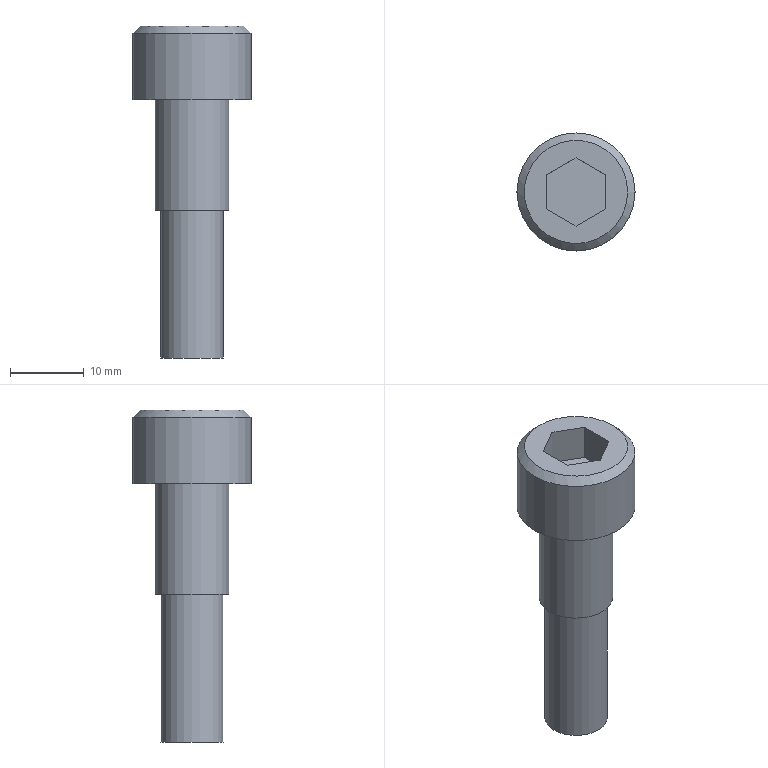Part | STEP file | M3-10_id1414_x_t | 1 solid | 15 faces | box 16 x 16 x 45 mm | volume 4022 mm3 | plane 11 | cylinder 3 | cone 1 | commonest cylinder face diameters 8.5 x1 10 x1 16 x1
STEP:
#1=CARTESIAN_POINT('',(-356.75,-267.5,-47.));
#2=VERTEX_POINT('',#1);
#3=CARTESIAN_POINT('',(-352.5,-267.5,-47.));
#4=DIRECTION('',(0.,0.,-1.));
#5=DIRECTION('',(-1.,0.,0.));
#6=AXIS2_PLACEMENT_3D('',#3,#4,#5);
#7=CIRCLE('',#6,4.25);
#8=EDGE_CURVE('',#2,#2,#7,.T.);
#9=ORIENTED_EDGE('',*,*,#8,.F.);
#10=EDGE_LOOP('',(#9));
#11=FACE_BOUND('',#10,.T.);
#12=CARTESIAN_POINT('',(-347.5,-267.5,-47.));
#13=VERTEX_POINT('',#12);
#14=CARTESIAN_POINT('',(-352.5,-267.5,-47.));
#15=DIRECTION('',(0.,0.,1.));
#16=DIRECTION('',(1.,0.,0.));
#17=AXIS2_PLACEMENT_3D('',#14,#15,#16);
#18=CIRCLE('',#17,5.);
#19=EDGE_CURVE('',#13,#13,#18,.T.);
#20=ORIENTED_EDGE('',*,*,#19,.F.);
#21=EDGE_LOOP('',(#20));
#22=FACE_BOUND('',#21,.T.);
#23=CARTESIAN_POINT('',(-352.5,-267.5,-47.));
#24=DIRECTION('',(0.,0.,-1.));
#25=DIRECTION('',(-1.,0.,0.));
#26=AXIS2_PLACEMENT_3D('',#23,#24,#25);
#27=PLANE('',#26);
#28=ADVANCED_FACE('',(#11,#22),#27,.T.);
#29=CARTESIAN_POINT('',(-357.5,-267.5,-32.));
#30=VERTEX_POINT('',#29);
#31=CARTESIAN_POINT('',(-352.5,-267.5,-32.));
#32=DIRECTION('',(0.,0.,1.));
#33=DIRECTION('',(-1.,0.,0.));
#34=AXIS2_PLACEMENT_3D('',#31,#32,#33);
#35=CIRCLE('',#34,5.);
#36=EDGE_CURVE('',#30,#30,#35,.T.);
#37=ORIENTED_EDGE('',*,*,#36,.F.);
#38=EDGE_LOOP('',(#37));
#39=FACE_BOUND('',#38,.T.);
#40=ORIENTED_EDGE('',*,*,#19,.T.);
#41=EDGE_LOOP('',(#40));
#42=FACE_BOUND('',#41,.T.);
#43=CARTESIAN_POINT('',(-352.5,-267.5,-47.));
#44=DIRECTION('',(0.,0.,1.));
#45=DIRECTION('',(1.,0.,0.));
#46=AXIS2_PLACEMENT_3D('',#43,#44,#45);
#47=CYLINDRICAL_SURFACE('',#46,5.);
#48=ADVANCED_FACE('',(#39,#42),#47,.T.);
#49=CARTESIAN_POINT('',(-348.25,-267.5,-67.));
#50=VERTEX_POINT('',#49);
#51=CARTESIAN_POINT('',(-352.5,-267.5,-67.));
#52=DIRECTION('',(0.,0.,1.));
#53=DIRECTION('',(1.,0.,0.));
#54=AXIS2_PLACEMENT_3D('',#51,#52,#53);
#55=CIRCLE('',#54,4.25);
#56=EDGE_CURVE('',#50,#50,#55,.T.);
#57=ORIENTED_EDGE('',*,*,#56,.F.);
#58=EDGE_LOOP('',(#57));
#59=FACE_OUTER_BOUND('',#58,.T.);
#60=CARTESIAN_POINT('',(-352.5,-267.5,-67.));
#61=DIRECTION('',(0.,0.,-1.));
#62=DIRECTION('',(-1.,0.,0.));
#63=AXIS2_PLACEMENT_3D('',#60,#61,#62);
#64=PLANE('',#63);
#65=ADVANCED_FACE('',(#59),#64,.T.);
#66=ORIENTED_EDGE('',*,*,#56,.T.);
#67=EDGE_LOOP('',(#66));
#68=FACE_BOUND('',#67,.T.);
#69=ORIENTED_EDGE('',*,*,#8,.T.);
#70=EDGE_LOOP('',(#69));
#71=FACE_BOUND('',#70,.T.);
#72=CARTESIAN_POINT('',(-352.5,-267.5,-47.));
#73=DIRECTION('',(0.,0.,-1.));
#74=DIRECTION('',(1.,0.,0.));
#75=AXIS2_PLACEMENT_3D('',#72,#73,#74);
#76=CYLINDRICAL_SURFACE('',#75,4.25);
#77=ADVANCED_FACE('',(#68,#71),#76,.T.);
#78=CARTESIAN_POINT('',(-356.5,-265.191,-22.));
#79=VERTEX_POINT('',#78);
#80=CARTESIAN_POINT('',(-356.5,-269.809,-22.));
#81=VERTEX_POINT('',#80);
#82=CARTESIAN_POINT('',(-356.5,-265.191,-22.));
#83=DIRECTION('',(0.,-1.,0.));
#84=VECTOR('',#83,1.);
#85=LINE('',#82,#84);
#86=EDGE_CURVE('',#79,#81,#85,.T.);
#87=ORIENTED_EDGE('',*,*,#86,.F.);
#88=CARTESIAN_POINT('',(-352.5,-262.881,-22.));
#89=VERTEX_POINT('',#88);
#90=CARTESIAN_POINT('',(-352.5,-262.881,-22.));
#91=DIRECTION('',(-0.866,-0.5,0.));
#92=VECTOR('',#91,1.);
#93=LINE('',#90,#92);
#94=EDGE_CURVE('',#89,#79,#93,.T.);
#95=ORIENTED_EDGE('',*,*,#94,.F.);
#96=CARTESIAN_POINT('',(-348.5,-265.191,-22.));
#97=VERTEX_POINT('',#96);
#98=CARTESIAN_POINT('',(-348.5,-265.191,-22.));
#99=DIRECTION('',(-0.866,0.5,0.));
#100=VECTOR('',#99,1.);
#101=LINE('',#98,#100);
#102=EDGE_CURVE('',#97,#89,#101,.T.);
#103=ORIENTED_EDGE('',*,*,#102,.F.);
#104=CARTESIAN_POINT('',(-348.5,-269.809,-22.));
#105=VERTEX_POINT('',#104);
#106=CARTESIAN_POINT('',(-348.5,-269.809,-22.));
#107=DIRECTION('',(0.,1.,0.));
#108=VECTOR('',#107,1.);
#109=LINE('',#106,#108);
#110=EDGE_CURVE('',#105,#97,#109,.T.);
#111=ORIENTED_EDGE('',*,*,#110,.F.);
#112=CARTESIAN_POINT('',(-352.5,-272.119,-22.));
#113=VERTEX_POINT('',#112);
#114=CARTESIAN_POINT('',(-352.5,-272.119,-22.));
#115=DIRECTION('',(0.866,0.5,0.));
#116=VECTOR('',#115,1.);
#117=LINE('',#114,#116);
#118=EDGE_CURVE('',#113,#105,#117,.T.);
#119=ORIENTED_EDGE('',*,*,#118,.F.);
#120=CARTESIAN_POINT('',(-356.5,-269.809,-22.));
#121=DIRECTION('',(0.866,-0.5,0.));
#122=VECTOR('',#121,1.);
#123=LINE('',#120,#122);
#124=EDGE_CURVE('',#81,#113,#123,.T.);
#125=ORIENTED_EDGE('',*,*,#124,.F.);
#126=EDGE_LOOP('',(#87,#95,#103,#111,#119,#125));
#127=FACE_BOUND('',#126,.T.);
#128=CARTESIAN_POINT('',(-345.5,-267.5,-22.));
#129=VERTEX_POINT('',#128);
#130=CARTESIAN_POINT('',(-352.5,-267.5,-22.));
#131=DIRECTION('',(0.,0.,1.));
#132=DIRECTION('',(1.,0.,0.));
#133=AXIS2_PLACEMENT_3D('',#130,#131,#132);
#134=CIRCLE('',#133,7.);
#135=EDGE_CURVE('',#129,#129,#134,.T.);
#136=ORIENTED_EDGE('',*,*,#135,.T.);
#137=EDGE_LOOP('',(#136));
#138=FACE_BOUND('',#137,.T.);
#139=CARTESIAN_POINT('',(-352.5,-267.5,-22.));
#140=DIRECTION('',(0.,0.,1.));
#141=DIRECTION('',(1.,0.,0.));
#142=AXIS2_PLACEMENT_3D('',#139,#140,#141);
#143=PLANE('',#142);
#144=ADVANCED_FACE('',(#127,#138),#143,.T.);
#145=ORIENTED_EDGE('',*,*,#36,.T.);
#146=EDGE_LOOP('',(#145));
#147=FACE_BOUND('',#146,.T.);
#148=CARTESIAN_POINT('',(-344.5,-267.5,-32.));
#149=VERTEX_POINT('',#148);
#150=CARTESIAN_POINT('',(-352.5,-267.5,-32.));
#151=DIRECTION('',(0.,0.,1.));
#152=DIRECTION('',(1.,0.,0.));
#153=AXIS2_PLACEMENT_3D('',#150,#151,#152);
#154=CIRCLE('',#153,8.);
#155=EDGE_CURVE('',#149,#149,#154,.T.);
#156=ORIENTED_EDGE('',*,*,#155,.F.);
#157=EDGE_LOOP('',(#156));
#158=FACE_BOUND('',#157,.T.);
#159=CARTESIAN_POINT('',(-352.5,-267.5,-32.));
#160=DIRECTION('',(0.,0.,-1.));
#161=DIRECTION('',(-1.,0.,0.));
#162=AXIS2_PLACEMENT_3D('',#159,#160,#161);
#163=PLANE('',#162);
#164=ADVANCED_FACE('',(#147,#158),#163,.T.);
#165=CARTESIAN_POINT('',(-344.5,-267.5,-23.));
#166=VERTEX_POINT('',#165);
#167=CARTESIAN_POINT('',(-352.5,-267.5,-23.));
#168=DIRECTION('',(0.,0.,-1.));
#169=DIRECTION('',(1.,0.,0.));
#170=AXIS2_PLACEMENT_3D('',#167,#168,#169);
#171=CIRCLE('',#170,8.);
#172=EDGE_CURVE('',#166,#166,#171,.T.);
#173=ORIENTED_EDGE('',*,*,#172,.T.);
#174=EDGE_LOOP('',(#173));
#175=FACE_BOUND('',#174,.T.);
#176=ORIENTED_EDGE('',*,*,#155,.T.);
#177=EDGE_LOOP('',(#176));
#178=FACE_BOUND('',#177,.T.);
#179=CARTESIAN_POINT('',(-352.5,-267.5,-32.));
#180=DIRECTION('',(0.,0.,1.));
#181=DIRECTION('',(1.,0.,0.));
#182=AXIS2_PLACEMENT_3D('',#179,#180,#181);
#183=CYLINDRICAL_SURFACE('',#182,8.);
#184=ADVANCED_FACE('',(#175,#178),#183,.T.);
#185=ORIENTED_EDGE('',*,*,#135,.F.);
#186=EDGE_LOOP('',(#185));
#187=FACE_BOUND('',#186,.T.);
#188=ORIENTED_EDGE('',*,*,#172,.F.);
#189=EDGE_LOOP('',(#188));
#190=FACE_BOUND('',#189,.T.);
#191=CARTESIAN_POINT('',(-352.5,-267.5,-23.));
#192=DIRECTION('',(0.,0.,-1.));
#193=DIRECTION('',(-1.,0.,0.));
#194=AXIS2_PLACEMENT_3D('',#191,#192,#193);
#195=CONICAL_SURFACE('',#194,8.,45.);
#196=ADVANCED_FACE('',(#187,#190),#195,.T.);
#197=ORIENTED_EDGE('',*,*,#86,.T.);
#198=CARTESIAN_POINT('',(-356.5,-269.809,-27.));
#199=VERTEX_POINT('',#198);
#200=CARTESIAN_POINT('',(-356.5,-269.809,-27.));
#201=DIRECTION('',(0.,0.,-1.));
#202=VECTOR('',#201,1.);
#203=LINE('',#200,#202);
#204=EDGE_CURVE('',#81,#199,#203,.T.);
#205=ORIENTED_EDGE('',*,*,#204,.T.);
#206=CARTESIAN_POINT('',(-356.5,-265.191,-27.));
#207=VERTEX_POINT('',#206);
#208=CARTESIAN_POINT('',(-356.5,-265.191,-27.));
#209=DIRECTION('',(0.,1.,0.));
#210=VECTOR('',#209,1.);
#211=LINE('',#208,#210);
#212=EDGE_CURVE('',#199,#207,#211,.T.);
#213=ORIENTED_EDGE('',*,*,#212,.T.);
#214=CARTESIAN_POINT('',(-356.5,-265.191,-27.));
#215=DIRECTION('',(0.,0.,-1.));
#216=VECTOR('',#215,1.);
#217=LINE('',#214,#216);
#218=EDGE_CURVE('',#79,#207,#217,.T.);
#219=ORIENTED_EDGE('',*,*,#218,.F.);
#220=EDGE_LOOP('',(#197,#205,#213,#219));
#221=FACE_OUTER_BOUND('',#220,.T.);
#222=CARTESIAN_POINT('',(-356.5,-265.191,-27.));
#223=DIRECTION('',(-1.,0.,0.));
#224=DIRECTION('',(0.,-1.,0.));
#225=AXIS2_PLACEMENT_3D('',#222,#223,#224);
#226=PLANE('',#225);
#227=ADVANCED_FACE('',(#221),#226,.F.);
#228=ORIENTED_EDGE('',*,*,#124,.T.);
#229=CARTESIAN_POINT('',(-352.5,-272.119,-27.));
#230=VERTEX_POINT('',#229);
#231=CARTESIAN_POINT('',(-352.5,-272.119,-27.));
#232=DIRECTION('',(0.,0.,-1.));
#233=VECTOR('',#232,1.);
#234=LINE('',#231,#233);
#235=EDGE_CURVE('',#113,#230,#234,.T.);
#236=ORIENTED_EDGE('',*,*,#235,.T.);
#237=CARTESIAN_POINT('',(-356.5,-269.809,-27.));
#238=DIRECTION('',(-0.866,0.5,0.));
#239=VECTOR('',#238,1.);
#240=LINE('',#237,#239);
#241=EDGE_CURVE('',#230,#199,#240,.T.);
#242=ORIENTED_EDGE('',*,*,#241,.T.);
#243=ORIENTED_EDGE('',*,*,#204,.F.);
#244=EDGE_LOOP('',(#228,#236,#242,#243));
#245=FACE_OUTER_BOUND('',#244,.T.);
#246=CARTESIAN_POINT('',(-356.5,-269.809,-27.));
#247=DIRECTION('',(-0.5,-0.866,0.));
#248=DIRECTION('',(0.866,-0.5,0.));
#249=AXIS2_PLACEMENT_3D('',#246,#247,#248);
#250=PLANE('',#249);
#251=ADVANCED_FACE('',(#245),#250,.F.);
#252=ORIENTED_EDGE('',*,*,#118,.T.);
#253=CARTESIAN_POINT('',(-348.5,-269.809,-27.));
#254=VERTEX_POINT('',#253);
#255=CARTESIAN_POINT('',(-348.5,-269.809,-27.));
#256=DIRECTION('',(0.,0.,-1.));
#257=VECTOR('',#256,1.);
#258=LINE('',#255,#257);
#259=EDGE_CURVE('',#105,#254,#258,.T.);
#260=ORIENTED_EDGE('',*,*,#259,.T.);
#261=CARTESIAN_POINT('',(-352.5,-272.119,-27.));
#262=DIRECTION('',(-0.866,-0.5,0.));
#263=VECTOR('',#262,1.);
#264=LINE('',#261,#263);
#265=EDGE_CURVE('',#254,#230,#264,.T.);
#266=ORIENTED_EDGE('',*,*,#265,.T.);
#267=ORIENTED_EDGE('',*,*,#235,.F.);
#268=EDGE_LOOP('',(#252,#260,#266,#267));
#269=FACE_OUTER_BOUND('',#268,.T.);
#270=CARTESIAN_POINT('',(-352.5,-272.119,-27.));
#271=DIRECTION('',(0.5,-0.866,0.));
#272=DIRECTION('',(0.866,0.5,0.));
#273=AXIS2_PLACEMENT_3D('',#270,#271,#272);
#274=PLANE('',#273);
#275=ADVANCED_FACE('',(#269),#274,.F.);
#276=ORIENTED_EDGE('',*,*,#110,.T.);
#277=CARTESIAN_POINT('',(-348.5,-265.191,-27.));
#278=VERTEX_POINT('',#277);
#279=CARTESIAN_POINT('',(-348.5,-265.191,-27.));
#280=DIRECTION('',(0.,0.,-1.));
#281=VECTOR('',#280,1.);
#282=LINE('',#279,#281);
#283=EDGE_CURVE('',#97,#278,#282,.T.);
#284=ORIENTED_EDGE('',*,*,#283,.T.);
#285=CARTESIAN_POINT('',(-348.5,-269.809,-27.));
#286=DIRECTION('',(0.,-1.,0.));
#287=VECTOR('',#286,1.);
#288=LINE('',#285,#287);
#289=EDGE_CURVE('',#278,#254,#288,.T.);
#290=ORIENTED_EDGE('',*,*,#289,.T.);
#291=ORIENTED_EDGE('',*,*,#259,.F.);
#292=EDGE_LOOP('',(#276,#284,#290,#291));
#293=FACE_OUTER_BOUND('',#292,.T.);
#294=CARTESIAN_POINT('',(-348.5,-269.809,-27.));
#295=DIRECTION('',(1.,0.,0.));
#296=DIRECTION('',(0.,1.,0.));
#297=AXIS2_PLACEMENT_3D('',#294,#295,#296);
#298=PLANE('',#297);
#299=ADVANCED_FACE('',(#293),#298,.F.);
#300=ORIENTED_EDGE('',*,*,#102,.T.);
#301=CARTESIAN_POINT('',(-352.5,-262.881,-27.));
#302=VERTEX_POINT('',#301);
#303=CARTESIAN_POINT('',(-352.5,-262.881,-27.));
#304=DIRECTION('',(0.,0.,-1.));
#305=VECTOR('',#304,1.);
#306=LINE('',#303,#305);
#307=EDGE_CURVE('',#89,#302,#306,.T.);
#308=ORIENTED_EDGE('',*,*,#307,.T.);
#309=CARTESIAN_POINT('',(-348.5,-265.191,-27.));
#310=DIRECTION('',(0.866,-0.5,0.));
#311=VECTOR('',#310,1.);
#312=LINE('',#309,#311);
#313=EDGE_CURVE('',#302,#278,#312,.T.);
#314=ORIENTED_EDGE('',*,*,#313,.T.);
#315=ORIENTED_EDGE('',*,*,#283,.F.);
#316=EDGE_LOOP('',(#300,#308,#314,#315));
#317=FACE_OUTER_BOUND('',#316,.T.);
#318=CARTESIAN_POINT('',(-348.5,-265.191,-27.));
#319=DIRECTION('',(0.5,0.866,0.));
#320=DIRECTION('',(-0.866,0.5,0.));
#321=AXIS2_PLACEMENT_3D('',#318,#319,#320);
#322=PLANE('',#321);
#323=ADVANCED_FACE('',(#317),#322,.F.);
#324=ORIENTED_EDGE('',*,*,#94,.T.);
#325=ORIENTED_EDGE('',*,*,#218,.T.);
#326=CARTESIAN_POINT('',(-352.5,-262.881,-27.));
#327=DIRECTION('',(0.866,0.5,0.));
#328=VECTOR('',#327,1.);
#329=LINE('',#326,#328);
#330=EDGE_CURVE('',#207,#302,#329,.T.);
#331=ORIENTED_EDGE('',*,*,#330,.T.);
#332=ORIENTED_EDGE('',*,*,#307,.F.);
#333=EDGE_LOOP('',(#324,#325,#331,#332));
#334=FACE_OUTER_BOUND('',#333,.T.);
#335=CARTESIAN_POINT('',(-352.5,-262.881,-27.));
#336=DIRECTION('',(-0.5,0.866,0.));
#337=DIRECTION('',(-0.866,-0.5,0.));
#338=AXIS2_PLACEMENT_3D('',#335,#336,#337);
#339=PLANE('',#338);
#340=ADVANCED_FACE('',(#334),#339,.F.);
#341=ORIENTED_EDGE('',*,*,#212,.F.);
#342=ORIENTED_EDGE('',*,*,#241,.F.);
#343=ORIENTED_EDGE('',*,*,#265,.F.);
#344=ORIENTED_EDGE('',*,*,#289,.F.);
#345=ORIENTED_EDGE('',*,*,#313,.F.);
#346=ORIENTED_EDGE('',*,*,#330,.F.);
#347=EDGE_LOOP('',(#341,#342,#343,#344,#345,#346));
#348=FACE_OUTER_BOUND('',#347,.T.);
#349=CARTESIAN_POINT('',(-352.5,-267.5,-27.));
#350=DIRECTION('',(0.,0.,1.));
#351=DIRECTION('',(1.,0.,0.));
#352=AXIS2_PLACEMENT_3D('',#349,#350,#351);
#353=PLANE('',#352);
#354=ADVANCED_FACE('',(#348),#353,.T.);
#355=CLOSED_SHELL('',(#28,#48,#65,#77,#144,#164,#184,#196,#227,#251,#275,#299,#323,#340,#354));
#356=MANIFOLD_SOLID_BREP('',#355);
#357=(LENGTH_UNIT()NAMED_UNIT(*)SI_UNIT(.MILLI.,.METRE.));
#358=UNCERTAINTY_MEASURE_WITH_UNIT(LENGTH_MEASURE(0.00002),#357,'','');
#359=(NAMED_UNIT(*)PLANE_ANGLE_UNIT()SI_UNIT($,.RADIAN.));
#360=PLANE_ANGLE_MEASURE_WITH_UNIT(PLANE_ANGLE_MEASURE(0.01745),#359);
#361=DIMENSIONAL_EXPONENTS(0.,0.,0.,0.,0.,0.,0.);
#362=(CONVERSION_BASED_UNIT('DEGREE',#360)NAMED_UNIT(#361)PLANE_ANGLE_UNIT());
#363=(NAMED_UNIT(*)SI_UNIT($,.STERADIAN.)SOLID_ANGLE_UNIT());
#364=(GEOMETRIC_REPRESENTATION_CONTEXT(3)GLOBAL_UNCERTAINTY_ASSIGNED_CONTEXT((#358))GLOBAL_UNIT_ASSIGNED_CONTEXT((#357,#362,#363))REPRESENTATION_CONTEXT('',''));
#365=ADVANCED_BREP_SHAPE_REPRESENTATION('',(#356),#364);